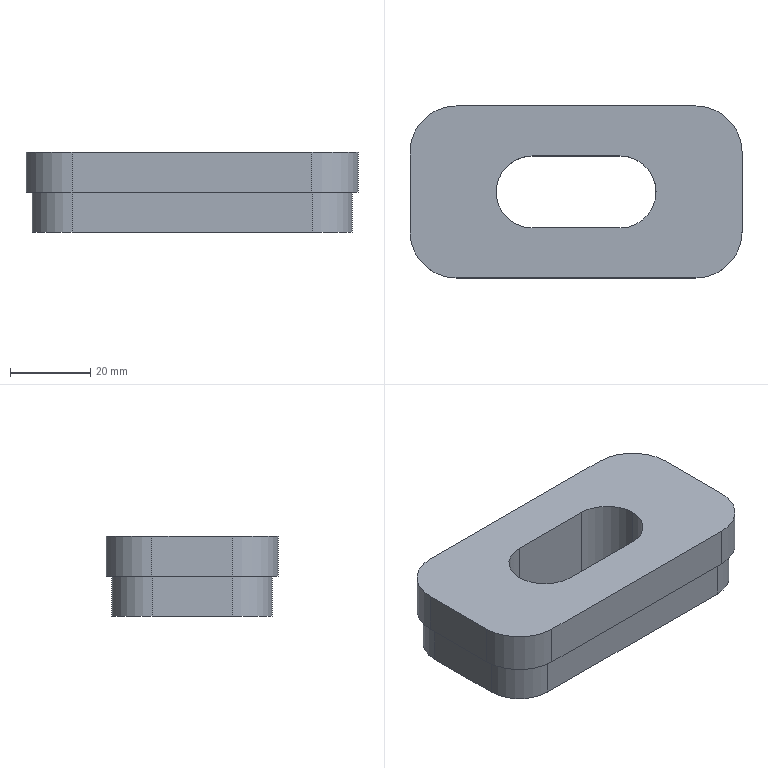Part | SolidWorks | features BaseBody 1 | 1 solid | 24 faces | box 83 x 43 x 20 mm | volume 52687 mm3 | plane 13 | cylinder 11 | commonest cylinder face diameters 20 x4 23 x4 18 x3
STEP:
#1=CARTESIAN_POINT('',(20.,0.,0.));
#2=VERTEX_POINT('',#1);
#3=CARTESIAN_POINT('',(11.,9.,0.));
#4=VERTEX_POINT('',#3);
#5=CARTESIAN_POINT('',(11.,0.,0.));
#6=DIRECTION('',(0.,0.,1.));
#7=DIRECTION('',(1.,0.,0.));
#8=AXIS2_PLACEMENT_3D('',#5,#6,#7);
#9=CIRCLE('',#8,9.);
#10=EDGE_CURVE('',#2,#4,#9,.T.);
#11=ORIENTED_EDGE('',*,*,#10,.F.);
#12=CARTESIAN_POINT('',(20.,0.,20.));
#13=VERTEX_POINT('',#12);
#14=CARTESIAN_POINT('',(20.,0.,0.));
#15=DIRECTION('',(0.,0.,1.));
#16=VECTOR('',#15,1000.);
#17=LINE('',#14,#16);
#18=EDGE_CURVE('',#2,#13,#17,.T.);
#19=ORIENTED_EDGE('',*,*,#18,.T.);
#20=CARTESIAN_POINT('',(11.,9.,20.));
#21=VERTEX_POINT('',#20);
#22=CARTESIAN_POINT('',(11.,0.,20.));
#23=DIRECTION('',(0.,0.,-1.));
#24=DIRECTION('',(1.,0.,0.));
#25=AXIS2_PLACEMENT_3D('',#22,#23,#24);
#26=CIRCLE('',#25,9.);
#27=EDGE_CURVE('',#21,#13,#26,.T.);
#28=ORIENTED_EDGE('',*,*,#27,.F.);
#29=CARTESIAN_POINT('',(11.,9.,0.));
#30=DIRECTION('',(0.,0.,1.));
#31=VECTOR('',#30,1000.);
#32=LINE('',#29,#31);
#33=EDGE_CURVE('',#4,#21,#32,.T.);
#34=ORIENTED_EDGE('',*,*,#33,.F.);
#35=EDGE_LOOP('',(#11,#19,#28,#34));
#36=FACE_OUTER_BOUND('',#35,.T.);
#37=CARTESIAN_POINT('',(11.,0.,0.));
#38=DIRECTION('',(0.,0.,1.));
#39=DIRECTION('',(1.,0.,0.));
#40=AXIS2_PLACEMENT_3D('',#37,#38,#39);
#41=CYLINDRICAL_SURFACE('',#40,9.);
#42=ADVANCED_FACE('',(#36),#41,.F.);
#43=CARTESIAN_POINT('',(11.,-9.,20.));
#44=VERTEX_POINT('',#43);
#45=CARTESIAN_POINT('',(-11.,-9.,20.));
#46=VERTEX_POINT('',#45);
#47=CARTESIAN_POINT('',(0.,-9.,20.));
#48=DIRECTION('',(-1.,0.,0.));
#49=VECTOR('',#48,1000.);
#50=LINE('',#47,#49);
#51=EDGE_CURVE('',#44,#46,#50,.T.);
#52=ORIENTED_EDGE('',*,*,#51,.T.);
#53=CARTESIAN_POINT('',(-11.,9.,20.));
#54=VERTEX_POINT('',#53);
#55=CARTESIAN_POINT('',(-11.,0.,20.));
#56=DIRECTION('',(0.,0.,-1.));
#57=DIRECTION('',(1.,0.,0.));
#58=AXIS2_PLACEMENT_3D('',#55,#56,#57);
#59=CIRCLE('',#58,9.);
#60=EDGE_CURVE('',#46,#54,#59,.T.);
#61=ORIENTED_EDGE('',*,*,#60,.T.);
#62=CARTESIAN_POINT('',(0.,9.,20.));
#63=DIRECTION('',(1.,0.,0.));
#64=VECTOR('',#63,1000.);
#65=LINE('',#62,#64);
#66=EDGE_CURVE('',#54,#21,#65,.T.);
#67=ORIENTED_EDGE('',*,*,#66,.T.);
#68=ORIENTED_EDGE('',*,*,#27,.T.);
#69=CARTESIAN_POINT('',(11.,0.,20.));
#70=DIRECTION('',(0.,0.,-1.));
#71=DIRECTION('',(1.,0.,0.));
#72=AXIS2_PLACEMENT_3D('',#69,#70,#71);
#73=CIRCLE('',#72,9.);
#74=EDGE_CURVE('',#13,#44,#73,.T.);
#75=ORIENTED_EDGE('',*,*,#74,.T.);
#76=EDGE_LOOP('',(#52,#61,#67,#68,#75));
#77=FACE_BOUND('',#76,.T.);
#78=CARTESIAN_POINT('',(41.5,-10.,20.));
#79=VERTEX_POINT('',#78);
#80=CARTESIAN_POINT('',(41.5,10.,20.));
#81=VERTEX_POINT('',#80);
#82=CARTESIAN_POINT('',(41.5,0.,20.));
#83=DIRECTION('',(0.,1.,0.));
#84=VECTOR('',#83,1000.);
#85=LINE('',#82,#84);
#86=EDGE_CURVE('',#79,#81,#85,.T.);
#87=ORIENTED_EDGE('',*,*,#86,.T.);
#88=CARTESIAN_POINT('',(30.,21.5,20.));
#89=VERTEX_POINT('',#88);
#90=CARTESIAN_POINT('',(30.,10.,20.));
#91=DIRECTION('',(0.,0.,1.));
#92=DIRECTION('',(1.,0.,0.));
#93=AXIS2_PLACEMENT_3D('',#90,#91,#92);
#94=CIRCLE('',#93,11.5);
#95=EDGE_CURVE('',#81,#89,#94,.T.);
#96=ORIENTED_EDGE('',*,*,#95,.T.);
#97=CARTESIAN_POINT('',(-30.,21.5,20.));
#98=VERTEX_POINT('',#97);
#99=CARTESIAN_POINT('',(0.,21.5,20.));
#100=DIRECTION('',(-1.,0.,0.));
#101=VECTOR('',#100,1000.);
#102=LINE('',#99,#101);
#103=EDGE_CURVE('',#89,#98,#102,.T.);
#104=ORIENTED_EDGE('',*,*,#103,.T.);
#105=CARTESIAN_POINT('',(-41.5,10.,20.));
#106=VERTEX_POINT('',#105);
#107=CARTESIAN_POINT('',(-30.,10.,20.));
#108=DIRECTION('',(0.,0.,1.));
#109=DIRECTION('',(1.,0.,0.));
#110=AXIS2_PLACEMENT_3D('',#107,#108,#109);
#111=CIRCLE('',#110,11.5);
#112=EDGE_CURVE('',#98,#106,#111,.T.);
#113=ORIENTED_EDGE('',*,*,#112,.T.);
#114=CARTESIAN_POINT('',(-41.5,-10.,20.));
#115=VERTEX_POINT('',#114);
#116=CARTESIAN_POINT('',(-41.5,0.,20.));
#117=DIRECTION('',(0.,-1.,0.));
#118=VECTOR('',#117,1000.);
#119=LINE('',#116,#118);
#120=EDGE_CURVE('',#106,#115,#119,.T.);
#121=ORIENTED_EDGE('',*,*,#120,.T.);
#122=CARTESIAN_POINT('',(-30.,-21.5,20.));
#123=VERTEX_POINT('',#122);
#124=CARTESIAN_POINT('',(-30.,-10.,20.));
#125=DIRECTION('',(0.,0.,1.));
#126=DIRECTION('',(1.,0.,0.));
#127=AXIS2_PLACEMENT_3D('',#124,#125,#126);
#128=CIRCLE('',#127,11.5);
#129=EDGE_CURVE('',#115,#123,#128,.T.);
#130=ORIENTED_EDGE('',*,*,#129,.T.);
#131=CARTESIAN_POINT('',(30.,-21.5,20.));
#132=VERTEX_POINT('',#131);
#133=CARTESIAN_POINT('',(0.,-21.5,20.));
#134=DIRECTION('',(1.,0.,0.));
#135=VECTOR('',#134,1000.);
#136=LINE('',#133,#135);
#137=EDGE_CURVE('',#123,#132,#136,.T.);
#138=ORIENTED_EDGE('',*,*,#137,.T.);
#139=CARTESIAN_POINT('',(30.,-10.,20.));
#140=DIRECTION('',(0.,0.,1.));
#141=DIRECTION('',(1.,0.,0.));
#142=AXIS2_PLACEMENT_3D('',#139,#140,#141);
#143=CIRCLE('',#142,11.5);
#144=EDGE_CURVE('',#132,#79,#143,.T.);
#145=ORIENTED_EDGE('',*,*,#144,.T.);
#146=EDGE_LOOP('',(#87,#96,#104,#113,#121,#130,#138,#145));
#147=FACE_OUTER_BOUND('',#146,.T.);
#148=CARTESIAN_POINT('',(0.,0.,20.));
#149=DIRECTION('',(0.,0.,1.));
#150=DIRECTION('',(1.,0.,0.));
#151=AXIS2_PLACEMENT_3D('',#148,#149,#150);
#152=PLANE('',#151);
#153=ADVANCED_FACE('',(#77,#147),#152,.T.);
#154=CARTESIAN_POINT('',(-11.,9.,0.));
#155=VERTEX_POINT('',#154);
#156=CARTESIAN_POINT('',(-11.,9.,0.));
#157=DIRECTION('',(0.,0.,-1.));
#158=VECTOR('',#157,1000.);
#159=LINE('',#156,#158);
#160=EDGE_CURVE('',#54,#155,#159,.T.);
#161=ORIENTED_EDGE('',*,*,#160,.F.);
#162=ORIENTED_EDGE('',*,*,#60,.F.);
#163=CARTESIAN_POINT('',(-11.,-9.,0.));
#164=VERTEX_POINT('',#163);
#165=CARTESIAN_POINT('',(-11.,-9.,0.));
#166=DIRECTION('',(0.,0.,1.));
#167=VECTOR('',#166,1000.);
#168=LINE('',#165,#167);
#169=EDGE_CURVE('',#164,#46,#168,.T.);
#170=ORIENTED_EDGE('',*,*,#169,.F.);
#171=CARTESIAN_POINT('',(-11.,0.,0.));
#172=DIRECTION('',(0.,0.,1.));
#173=DIRECTION('',(1.,0.,0.));
#174=AXIS2_PLACEMENT_3D('',#171,#172,#173);
#175=CIRCLE('',#174,9.);
#176=EDGE_CURVE('',#155,#164,#175,.T.);
#177=ORIENTED_EDGE('',*,*,#176,.F.);
#178=EDGE_LOOP('',(#161,#162,#170,#177));
#179=FACE_OUTER_BOUND('',#178,.T.);
#180=CARTESIAN_POINT('',(-11.,0.,0.));
#181=DIRECTION('',(0.,0.,1.));
#182=DIRECTION('',(1.,0.,0.));
#183=AXIS2_PLACEMENT_3D('',#180,#181,#182);
#184=CYLINDRICAL_SURFACE('',#183,9.);
#185=ADVANCED_FACE('',(#179),#184,.F.);
#186=ORIENTED_EDGE('',*,*,#51,.F.);
#187=CARTESIAN_POINT('',(11.,-9.,0.));
#188=VERTEX_POINT('',#187);
#189=CARTESIAN_POINT('',(11.,-9.,9.25));
#190=DIRECTION('',(0.,0.,-1.));
#191=VECTOR('',#190,1000.);
#192=LINE('',#189,#191);
#193=EDGE_CURVE('',#44,#188,#192,.T.);
#194=ORIENTED_EDGE('',*,*,#193,.T.);
#195=CARTESIAN_POINT('',(0.,-9.,0.));
#196=DIRECTION('',(-1.,0.,0.));
#197=VECTOR('',#196,1000.);
#198=LINE('',#195,#197);
#199=EDGE_CURVE('',#188,#164,#198,.T.);
#200=ORIENTED_EDGE('',*,*,#199,.T.);
#201=ORIENTED_EDGE('',*,*,#169,.T.);
#202=EDGE_LOOP('',(#186,#194,#200,#201));
#203=FACE_OUTER_BOUND('',#202,.T.);
#204=CARTESIAN_POINT('',(0.,-9.,9.25));
#205=DIRECTION('',(0.,1.,0.));
#206=DIRECTION('',(0.,0.,1.));
#207=AXIS2_PLACEMENT_3D('',#204,#205,#206);
#208=PLANE('',#207);
#209=ADVANCED_FACE('',(#203),#208,.T.);
#210=ORIENTED_EDGE('',*,*,#18,.F.);
#211=CARTESIAN_POINT('',(11.,0.,0.));
#212=DIRECTION('',(0.,0.,1.));
#213=DIRECTION('',(1.,0.,0.));
#214=AXIS2_PLACEMENT_3D('',#211,#212,#213);
#215=CIRCLE('',#214,9.);
#216=EDGE_CURVE('',#188,#2,#215,.T.);
#217=ORIENTED_EDGE('',*,*,#216,.F.);
#218=ORIENTED_EDGE('',*,*,#193,.F.);
#219=ORIENTED_EDGE('',*,*,#74,.F.);
#220=EDGE_LOOP('',(#210,#217,#218,#219));
#221=FACE_OUTER_BOUND('',#220,.T.);
#222=CARTESIAN_POINT('',(11.,0.,0.));
#223=DIRECTION('',(0.,0.,1.));
#224=DIRECTION('',(1.,0.,0.));
#225=AXIS2_PLACEMENT_3D('',#222,#223,#224);
#226=CYLINDRICAL_SURFACE('',#225,9.);
#227=ADVANCED_FACE('',(#221),#226,.F.);
#228=ORIENTED_EDGE('',*,*,#33,.T.);
#229=ORIENTED_EDGE('',*,*,#66,.F.);
#230=ORIENTED_EDGE('',*,*,#160,.T.);
#231=CARTESIAN_POINT('',(0.,9.,0.));
#232=DIRECTION('',(-1.,0.,0.));
#233=VECTOR('',#232,1000.);
#234=LINE('',#231,#233);
#235=EDGE_CURVE('',#4,#155,#234,.T.);
#236=ORIENTED_EDGE('',*,*,#235,.F.);
#237=EDGE_LOOP('',(#228,#229,#230,#236));
#238=FACE_OUTER_BOUND('',#237,.T.);
#239=CARTESIAN_POINT('',(0.,9.,9.25));
#240=DIRECTION('',(0.,1.,0.));
#241=DIRECTION('',(0.,0.,1.));
#242=AXIS2_PLACEMENT_3D('',#239,#240,#241);
#243=PLANE('',#242);
#244=ADVANCED_FACE('',(#238),#243,.F.);
#245=CARTESIAN_POINT('',(30.,21.5,10.));
#246=VERTEX_POINT('',#245);
#247=CARTESIAN_POINT('',(30.,21.5,10.));
#248=DIRECTION('',(0.,0.,1.));
#249=VECTOR('',#248,1000.);
#250=LINE('',#247,#249);
#251=EDGE_CURVE('',#246,#89,#250,.T.);
#252=ORIENTED_EDGE('',*,*,#251,.T.);
#253=ORIENTED_EDGE('',*,*,#95,.F.);
#254=CARTESIAN_POINT('',(41.5,10.,10.));
#255=VERTEX_POINT('',#254);
#256=CARTESIAN_POINT('',(41.5,10.,10.));
#257=DIRECTION('',(0.,0.,-1.));
#258=VECTOR('',#257,1000.);
#259=LINE('',#256,#258);
#260=EDGE_CURVE('',#81,#255,#259,.T.);
#261=ORIENTED_EDGE('',*,*,#260,.T.);
#262=CARTESIAN_POINT('',(30.,10.,10.));
#263=DIRECTION('',(0.,0.,1.));
#264=DIRECTION('',(1.,0.,0.));
#265=AXIS2_PLACEMENT_3D('',#262,#263,#264);
#266=CIRCLE('',#265,11.5);
#267=EDGE_CURVE('',#255,#246,#266,.T.);
#268=ORIENTED_EDGE('',*,*,#267,.T.);
#269=EDGE_LOOP('',(#252,#253,#261,#268));
#270=FACE_OUTER_BOUND('',#269,.T.);
#271=CARTESIAN_POINT('',(30.,10.,10.));
#272=DIRECTION('',(0.,0.,1.));
#273=DIRECTION('',(1.,0.,0.));
#274=AXIS2_PLACEMENT_3D('',#271,#272,#273);
#275=CYLINDRICAL_SURFACE('',#274,11.5);
#276=ADVANCED_FACE('',(#270),#275,.T.);
#277=ORIENTED_EDGE('',*,*,#260,.F.);
#278=ORIENTED_EDGE('',*,*,#86,.F.);
#279=CARTESIAN_POINT('',(41.5,-10.,10.));
#280=VERTEX_POINT('',#279);
#281=CARTESIAN_POINT('',(41.5,-10.,15.));
#282=DIRECTION('',(0.,0.,-1.));
#283=VECTOR('',#282,1000.);
#284=LINE('',#281,#283);
#285=EDGE_CURVE('',#79,#280,#284,.T.);
#286=ORIENTED_EDGE('',*,*,#285,.T.);
#287=CARTESIAN_POINT('',(41.5,0.,10.));
#288=DIRECTION('',(0.,1.,0.));
#289=VECTOR('',#288,1000.);
#290=LINE('',#287,#289);
#291=EDGE_CURVE('',#280,#255,#290,.T.);
#292=ORIENTED_EDGE('',*,*,#291,.T.);
#293=EDGE_LOOP('',(#277,#278,#286,#292));
#294=FACE_OUTER_BOUND('',#293,.T.);
#295=CARTESIAN_POINT('',(41.5,0.,15.));
#296=DIRECTION('',(1.,0.,0.));
#297=DIRECTION('',(0.,0.,-1.));
#298=AXIS2_PLACEMENT_3D('',#295,#296,#297);
#299=PLANE('',#298);
#300=ADVANCED_FACE('',(#294),#299,.T.);
#301=ORIENTED_EDGE('',*,*,#285,.F.);
#302=ORIENTED_EDGE('',*,*,#144,.F.);
#303=CARTESIAN_POINT('',(30.,-21.5,10.));
#304=VERTEX_POINT('',#303);
#305=CARTESIAN_POINT('',(30.,-21.5,10.));
#306=DIRECTION('',(0.,0.,-1.));
#307=VECTOR('',#306,1000.);
#308=LINE('',#305,#307);
#309=EDGE_CURVE('',#132,#304,#308,.T.);
#310=ORIENTED_EDGE('',*,*,#309,.T.);
#311=CARTESIAN_POINT('',(30.,-10.,10.));
#312=DIRECTION('',(0.,0.,1.));
#313=DIRECTION('',(1.,0.,0.));
#314=AXIS2_PLACEMENT_3D('',#311,#312,#313);
#315=CIRCLE('',#314,11.5);
#316=EDGE_CURVE('',#304,#280,#315,.T.);
#317=ORIENTED_EDGE('',*,*,#316,.T.);
#318=EDGE_LOOP('',(#301,#302,#310,#317));
#319=FACE_OUTER_BOUND('',#318,.T.);
#320=CARTESIAN_POINT('',(30.,-10.,10.));
#321=DIRECTION('',(0.,0.,1.));
#322=DIRECTION('',(1.,0.,0.));
#323=AXIS2_PLACEMENT_3D('',#320,#321,#322);
#324=CYLINDRICAL_SURFACE('',#323,11.5);
#325=ADVANCED_FACE('',(#319),#324,.T.);
#326=CARTESIAN_POINT('',(-30.,-21.5,10.));
#327=VERTEX_POINT('',#326);
#328=CARTESIAN_POINT('',(0.,-21.5,10.));
#329=DIRECTION('',(-1.,0.,0.));
#330=VECTOR('',#329,1000.);
#331=LINE('',#328,#330);
#332=EDGE_CURVE('',#304,#327,#331,.T.);
#333=ORIENTED_EDGE('',*,*,#332,.F.);
#334=ORIENTED_EDGE('',*,*,#309,.F.);
#335=ORIENTED_EDGE('',*,*,#137,.F.);
#336=CARTESIAN_POINT('',(-30.,-21.5,15.));
#337=DIRECTION('',(0.,0.,1.));
#338=VECTOR('',#337,1000.);
#339=LINE('',#336,#338);
#340=EDGE_CURVE('',#327,#123,#339,.T.);
#341=ORIENTED_EDGE('',*,*,#340,.F.);
#342=EDGE_LOOP('',(#333,#334,#335,#341));
#343=FACE_OUTER_BOUND('',#342,.T.);
#344=CARTESIAN_POINT('',(0.,-21.5,15.));
#345=DIRECTION('',(0.,1.,0.));
#346=DIRECTION('',(0.,0.,1.));
#347=AXIS2_PLACEMENT_3D('',#344,#345,#346);
#348=PLANE('',#347);
#349=ADVANCED_FACE('',(#343),#348,.F.);
#350=ORIENTED_EDGE('',*,*,#340,.T.);
#351=ORIENTED_EDGE('',*,*,#129,.F.);
#352=CARTESIAN_POINT('',(-41.5,-10.,10.));
#353=VERTEX_POINT('',#352);
#354=CARTESIAN_POINT('',(-41.5,-10.,10.));
#355=DIRECTION('',(0.,0.,-1.));
#356=VECTOR('',#355,1000.);
#357=LINE('',#354,#356);
#358=EDGE_CURVE('',#115,#353,#357,.T.);
#359=ORIENTED_EDGE('',*,*,#358,.T.);
#360=CARTESIAN_POINT('',(-30.,-10.,10.));
#361=DIRECTION('',(0.,0.,1.));
#362=DIRECTION('',(1.,0.,0.));
#363=AXIS2_PLACEMENT_3D('',#360,#361,#362);
#364=CIRCLE('',#363,11.5);
#365=EDGE_CURVE('',#353,#327,#364,.T.);
#366=ORIENTED_EDGE('',*,*,#365,.T.);
#367=EDGE_LOOP('',(#350,#351,#359,#366));
#368=FACE_OUTER_BOUND('',#367,.T.);
#369=CARTESIAN_POINT('',(-30.,-10.,10.));
#370=DIRECTION('',(0.,0.,1.));
#371=DIRECTION('',(1.,0.,0.));
#372=AXIS2_PLACEMENT_3D('',#369,#370,#371);
#373=CYLINDRICAL_SURFACE('',#372,11.5);
#374=ADVANCED_FACE('',(#368),#373,.T.);
#375=CARTESIAN_POINT('',(-41.5,10.,10.));
#376=VERTEX_POINT('',#375);
#377=CARTESIAN_POINT('',(-41.5,0.,10.));
#378=DIRECTION('',(0.,1.,0.));
#379=VECTOR('',#378,1000.);
#380=LINE('',#377,#379);
#381=EDGE_CURVE('',#353,#376,#380,.T.);
#382=ORIENTED_EDGE('',*,*,#381,.F.);
#383=ORIENTED_EDGE('',*,*,#358,.F.);
#384=ORIENTED_EDGE('',*,*,#120,.F.);
#385=CARTESIAN_POINT('',(-41.5,10.,15.));
#386=DIRECTION('',(0.,0.,1.));
#387=VECTOR('',#386,1000.);
#388=LINE('',#385,#387);
#389=EDGE_CURVE('',#376,#106,#388,.T.);
#390=ORIENTED_EDGE('',*,*,#389,.F.);
#391=EDGE_LOOP('',(#382,#383,#384,#390));
#392=FACE_OUTER_BOUND('',#391,.T.);
#393=CARTESIAN_POINT('',(-41.5,0.,15.));
#394=DIRECTION('',(1.,0.,0.));
#395=DIRECTION('',(0.,0.,-1.));
#396=AXIS2_PLACEMENT_3D('',#393,#394,#395);
#397=PLANE('',#396);
#398=ADVANCED_FACE('',(#392),#397,.F.);
#399=ORIENTED_EDGE('',*,*,#389,.T.);
#400=ORIENTED_EDGE('',*,*,#112,.F.);
#401=CARTESIAN_POINT('',(-30.,21.5,10.));
#402=VERTEX_POINT('',#401);
#403=CARTESIAN_POINT('',(-30.,21.5,10.));
#404=DIRECTION('',(0.,0.,-1.));
#405=VECTOR('',#404,1000.);
#406=LINE('',#403,#405);
#407=EDGE_CURVE('',#98,#402,#406,.T.);
#408=ORIENTED_EDGE('',*,*,#407,.T.);
#409=CARTESIAN_POINT('',(-30.,10.,10.));
#410=DIRECTION('',(0.,0.,1.));
#411=DIRECTION('',(1.,0.,0.));
#412=AXIS2_PLACEMENT_3D('',#409,#410,#411);
#413=CIRCLE('',#412,11.5);
#414=EDGE_CURVE('',#402,#376,#413,.T.);
#415=ORIENTED_EDGE('',*,*,#414,.T.);
#416=EDGE_LOOP('',(#399,#400,#408,#415));
#417=FACE_OUTER_BOUND('',#416,.T.);
#418=CARTESIAN_POINT('',(-30.,10.,10.));
#419=DIRECTION('',(0.,0.,1.));
#420=DIRECTION('',(1.,0.,0.));
#421=AXIS2_PLACEMENT_3D('',#418,#419,#420);
#422=CYLINDRICAL_SURFACE('',#421,11.5);
#423=ADVANCED_FACE('',(#417),#422,.T.);
#424=ORIENTED_EDGE('',*,*,#407,.F.);
#425=ORIENTED_EDGE('',*,*,#103,.F.);
#426=ORIENTED_EDGE('',*,*,#251,.F.);
#427=CARTESIAN_POINT('',(0.,21.5,10.));
#428=DIRECTION('',(-1.,0.,0.));
#429=VECTOR('',#428,1000.);
#430=LINE('',#427,#429);
#431=EDGE_CURVE('',#246,#402,#430,.T.);
#432=ORIENTED_EDGE('',*,*,#431,.T.);
#433=EDGE_LOOP('',(#424,#425,#426,#432));
#434=FACE_OUTER_BOUND('',#433,.T.);
#435=CARTESIAN_POINT('',(0.,21.5,15.));
#436=DIRECTION('',(0.,1.,0.));
#437=DIRECTION('',(0.,0.,1.));
#438=AXIS2_PLACEMENT_3D('',#435,#436,#437);
#439=PLANE('',#438);
#440=ADVANCED_FACE('',(#434),#439,.T.);
#441=ORIENTED_EDGE('',*,*,#216,.T.);
#442=ORIENTED_EDGE('',*,*,#10,.T.);
#443=ORIENTED_EDGE('',*,*,#235,.T.);
#444=ORIENTED_EDGE('',*,*,#176,.T.);
#445=ORIENTED_EDGE('',*,*,#199,.F.);
#446=EDGE_LOOP('',(#441,#442,#443,#444,#445));
#447=FACE_BOUND('',#446,.T.);
#448=CARTESIAN_POINT('',(30.,-20.,0.));
#449=VERTEX_POINT('',#448);
#450=CARTESIAN_POINT('',(40.,-10.,0.));
#451=VERTEX_POINT('',#450);
#452=CARTESIAN_POINT('',(30.,-10.,0.));
#453=DIRECTION('',(0.,0.,1.));
#454=DIRECTION('',(-1.,0.,0.));
#455=AXIS2_PLACEMENT_3D('',#452,#453,#454);
#456=CIRCLE('',#455,10.);
#457=EDGE_CURVE('',#449,#451,#456,.T.);
#458=ORIENTED_EDGE('',*,*,#457,.F.);
#459=CARTESIAN_POINT('',(-30.,-20.,0.));
#460=VERTEX_POINT('',#459);
#461=CARTESIAN_POINT('',(0.,-20.,0.));
#462=DIRECTION('',(1.,0.,0.));
#463=VECTOR('',#462,1000.);
#464=LINE('',#461,#463);
#465=EDGE_CURVE('',#460,#449,#464,.T.);
#466=ORIENTED_EDGE('',*,*,#465,.F.);
#467=CARTESIAN_POINT('',(-40.,-10.,0.));
#468=VERTEX_POINT('',#467);
#469=CARTESIAN_POINT('',(-30.,-10.,0.));
#470=DIRECTION('',(0.,0.,1.));
#471=DIRECTION('',(-1.,0.,0.));
#472=AXIS2_PLACEMENT_3D('',#469,#470,#471);
#473=CIRCLE('',#472,10.);
#474=EDGE_CURVE('',#468,#460,#473,.T.);
#475=ORIENTED_EDGE('',*,*,#474,.F.);
#476=CARTESIAN_POINT('',(-40.,10.,0.));
#477=VERTEX_POINT('',#476);
#478=CARTESIAN_POINT('',(-40.,0.,0.));
#479=DIRECTION('',(0.,-1.,0.));
#480=VECTOR('',#479,1000.);
#481=LINE('',#478,#480);
#482=EDGE_CURVE('',#477,#468,#481,.T.);
#483=ORIENTED_EDGE('',*,*,#482,.F.);
#484=CARTESIAN_POINT('',(-30.,20.,0.));
#485=VERTEX_POINT('',#484);
#486=CARTESIAN_POINT('',(-30.,10.,0.));
#487=DIRECTION('',(0.,0.,1.));
#488=DIRECTION('',(-1.,0.,0.));
#489=AXIS2_PLACEMENT_3D('',#486,#487,#488);
#490=CIRCLE('',#489,10.);
#491=EDGE_CURVE('',#485,#477,#490,.T.);
#492=ORIENTED_EDGE('',*,*,#491,.F.);
#493=CARTESIAN_POINT('',(30.,20.,0.));
#494=VERTEX_POINT('',#493);
#495=CARTESIAN_POINT('',(0.,20.,0.));
#496=DIRECTION('',(-1.,0.,0.));
#497=VECTOR('',#496,1000.);
#498=LINE('',#495,#497);
#499=EDGE_CURVE('',#494,#485,#498,.T.);
#500=ORIENTED_EDGE('',*,*,#499,.F.);
#501=CARTESIAN_POINT('',(40.,10.,0.));
#502=VERTEX_POINT('',#501);
#503=CARTESIAN_POINT('',(30.,10.,0.));
#504=DIRECTION('',(0.,0.,1.));
#505=DIRECTION('',(-1.,0.,0.));
#506=AXIS2_PLACEMENT_3D('',#503,#504,#505);
#507=CIRCLE('',#506,10.);
#508=EDGE_CURVE('',#502,#494,#507,.T.);
#509=ORIENTED_EDGE('',*,*,#508,.F.);
#510=CARTESIAN_POINT('',(40.,0.,0.));
#511=DIRECTION('',(0.,1.,0.));
#512=VECTOR('',#511,1000.);
#513=LINE('',#510,#512);
#514=EDGE_CURVE('',#451,#502,#513,.T.);
#515=ORIENTED_EDGE('',*,*,#514,.F.);
#516=EDGE_LOOP('',(#458,#466,#475,#483,#492,#500,#509,#515));
#517=FACE_OUTER_BOUND('',#516,.T.);
#518=CARTESIAN_POINT('',(0.,0.,0.));
#519=DIRECTION('',(0.,0.,1.));
#520=DIRECTION('',(1.,0.,0.));
#521=AXIS2_PLACEMENT_3D('',#518,#519,#520);
#522=PLANE('',#521);
#523=ADVANCED_FACE('',(#447,#517),#522,.F.);
#524=CARTESIAN_POINT('',(-40.,10.,10.));
#525=VERTEX_POINT('',#524);
#526=CARTESIAN_POINT('',(-30.,20.,10.));
#527=VERTEX_POINT('',#526);
#528=CARTESIAN_POINT('',(-30.,10.,10.));
#529=DIRECTION('',(0.,0.,-1.));
#530=DIRECTION('',(-1.,0.,0.));
#531=AXIS2_PLACEMENT_3D('',#528,#529,#530);
#532=CIRCLE('',#531,10.);
#533=EDGE_CURVE('',#525,#527,#532,.T.);
#534=ORIENTED_EDGE('',*,*,#533,.F.);
#535=CARTESIAN_POINT('',(-40.,-10.,10.));
#536=VERTEX_POINT('',#535);
#537=CARTESIAN_POINT('',(-40.,0.,10.));
#538=DIRECTION('',(0.,1.,0.));
#539=VECTOR('',#538,1000.);
#540=LINE('',#537,#539);
#541=EDGE_CURVE('',#536,#525,#540,.T.);
#542=ORIENTED_EDGE('',*,*,#541,.F.);
#543=CARTESIAN_POINT('',(-30.,-20.,10.));
#544=VERTEX_POINT('',#543);
#545=CARTESIAN_POINT('',(-30.,-10.,10.));
#546=DIRECTION('',(0.,0.,-1.));
#547=DIRECTION('',(-1.,0.,0.));
#548=AXIS2_PLACEMENT_3D('',#545,#546,#547);
#549=CIRCLE('',#548,10.);
#550=EDGE_CURVE('',#544,#536,#549,.T.);
#551=ORIENTED_EDGE('',*,*,#550,.F.);
#552=CARTESIAN_POINT('',(30.,-20.,10.));
#553=VERTEX_POINT('',#552);
#554=CARTESIAN_POINT('',(0.,-20.,10.));
#555=DIRECTION('',(-1.,0.,0.));
#556=VECTOR('',#555,1000.);
#557=LINE('',#554,#556);
#558=EDGE_CURVE('',#553,#544,#557,.T.);
#559=ORIENTED_EDGE('',*,*,#558,.F.);
#560=CARTESIAN_POINT('',(40.,-10.,10.));
#561=VERTEX_POINT('',#560);
#562=CARTESIAN_POINT('',(30.,-10.,10.));
#563=DIRECTION('',(0.,0.,-1.));
#564=DIRECTION('',(-1.,0.,0.));
#565=AXIS2_PLACEMENT_3D('',#562,#563,#564);
#566=CIRCLE('',#565,10.);
#567=EDGE_CURVE('',#561,#553,#566,.T.);
#568=ORIENTED_EDGE('',*,*,#567,.F.);
#569=CARTESIAN_POINT('',(40.,10.,10.));
#570=VERTEX_POINT('',#569);
#571=CARTESIAN_POINT('',(40.,0.,10.));
#572=DIRECTION('',(0.,-1.,0.));
#573=VECTOR('',#572,1000.);
#574=LINE('',#571,#573);
#575=EDGE_CURVE('',#570,#561,#574,.T.);
#576=ORIENTED_EDGE('',*,*,#575,.F.);
#577=CARTESIAN_POINT('',(30.,20.,10.));
#578=VERTEX_POINT('',#577);
#579=CARTESIAN_POINT('',(30.,10.,10.));
#580=DIRECTION('',(0.,0.,-1.));
#581=DIRECTION('',(-1.,0.,0.));
#582=AXIS2_PLACEMENT_3D('',#579,#580,#581);
#583=CIRCLE('',#582,10.);
#584=EDGE_CURVE('',#578,#570,#583,.T.);
#585=ORIENTED_EDGE('',*,*,#584,.F.);
#586=CARTESIAN_POINT('',(0.,20.,10.));
#587=DIRECTION('',(1.,0.,0.));
#588=VECTOR('',#587,1000.);
#589=LINE('',#586,#588);
#590=EDGE_CURVE('',#527,#578,#589,.T.);
#591=ORIENTED_EDGE('',*,*,#590,.F.);
#592=EDGE_LOOP('',(#534,#542,#551,#559,#568,#576,#585,#591));
#593=FACE_BOUND('',#592,.T.);
#594=ORIENTED_EDGE('',*,*,#291,.F.);
#595=ORIENTED_EDGE('',*,*,#316,.F.);
#596=ORIENTED_EDGE('',*,*,#332,.T.);
#597=ORIENTED_EDGE('',*,*,#365,.F.);
#598=ORIENTED_EDGE('',*,*,#381,.T.);
#599=ORIENTED_EDGE('',*,*,#414,.F.);
#600=ORIENTED_EDGE('',*,*,#431,.F.);
#601=ORIENTED_EDGE('',*,*,#267,.F.);
#602=EDGE_LOOP('',(#594,#595,#596,#597,#598,#599,#600,#601));
#603=FACE_OUTER_BOUND('',#602,.T.);
#604=CARTESIAN_POINT('',(0.,0.,10.));
#605=DIRECTION('',(0.,0.,1.));
#606=DIRECTION('',(1.,0.,0.));
#607=AXIS2_PLACEMENT_3D('',#604,#605,#606);
#608=PLANE('',#607);
#609=ADVANCED_FACE('',(#593,#603),#608,.F.);
#610=CARTESIAN_POINT('',(40.,10.,9.25));
#611=DIRECTION('',(0.,0.,1.));
#612=VECTOR('',#611,1000.);
#613=LINE('',#610,#612);
#614=EDGE_CURVE('',#502,#570,#613,.T.);
#615=ORIENTED_EDGE('',*,*,#614,.T.);
#616=ORIENTED_EDGE('',*,*,#575,.T.);
#617=CARTESIAN_POINT('',(40.,-10.,9.25));
#618=DIRECTION('',(0.,0.,-1.));
#619=VECTOR('',#618,1000.);
#620=LINE('',#617,#619);
#621=EDGE_CURVE('',#561,#451,#620,.T.);
#622=ORIENTED_EDGE('',*,*,#621,.T.);
#623=ORIENTED_EDGE('',*,*,#514,.T.);
#624=EDGE_LOOP('',(#615,#616,#622,#623));
#625=FACE_OUTER_BOUND('',#624,.T.);
#626=CARTESIAN_POINT('',(40.,0.,9.25));
#627=DIRECTION('',(1.,0.,0.));
#628=DIRECTION('',(0.,0.,-1.));
#629=AXIS2_PLACEMENT_3D('',#626,#627,#628);
#630=PLANE('',#629);
#631=ADVANCED_FACE('',(#625),#630,.T.);
#632=ORIENTED_EDGE('',*,*,#621,.F.);
#633=ORIENTED_EDGE('',*,*,#567,.T.);
#634=CARTESIAN_POINT('',(30.,-20.,18.5));
#635=DIRECTION('',(0.,0.,-1.));
#636=VECTOR('',#635,1000.);
#637=LINE('',#634,#636);
#638=EDGE_CURVE('',#553,#449,#637,.T.);
#639=ORIENTED_EDGE('',*,*,#638,.T.);
#640=ORIENTED_EDGE('',*,*,#457,.T.);
#641=EDGE_LOOP('',(#632,#633,#639,#640));
#642=FACE_OUTER_BOUND('',#641,.T.);
#643=CARTESIAN_POINT('',(30.,-10.,18.5));
#644=DIRECTION('',(0.,0.,-1.));
#645=DIRECTION('',(-1.,0.,0.));
#646=AXIS2_PLACEMENT_3D('',#643,#644,#645);
#647=CYLINDRICAL_SURFACE('',#646,10.);
#648=ADVANCED_FACE('',(#642),#647,.T.);
#649=ORIENTED_EDGE('',*,*,#465,.T.);
#650=ORIENTED_EDGE('',*,*,#638,.F.);
#651=ORIENTED_EDGE('',*,*,#558,.T.);
#652=CARTESIAN_POINT('',(-30.,-20.,9.25));
#653=DIRECTION('',(0.,0.,1.));
#654=VECTOR('',#653,1000.);
#655=LINE('',#652,#654);
#656=EDGE_CURVE('',#460,#544,#655,.T.);
#657=ORIENTED_EDGE('',*,*,#656,.F.);
#658=EDGE_LOOP('',(#649,#650,#651,#657));
#659=FACE_OUTER_BOUND('',#658,.T.);
#660=CARTESIAN_POINT('',(0.,-20.,9.25));
#661=DIRECTION('',(0.,1.,0.));
#662=DIRECTION('',(0.,0.,1.));
#663=AXIS2_PLACEMENT_3D('',#660,#661,#662);
#664=PLANE('',#663);
#665=ADVANCED_FACE('',(#659),#664,.F.);
#666=ORIENTED_EDGE('',*,*,#656,.T.);
#667=ORIENTED_EDGE('',*,*,#550,.T.);
#668=CARTESIAN_POINT('',(-40.,-10.,18.5));
#669=DIRECTION('',(0.,0.,-1.));
#670=VECTOR('',#669,1000.);
#671=LINE('',#668,#670);
#672=EDGE_CURVE('',#536,#468,#671,.T.);
#673=ORIENTED_EDGE('',*,*,#672,.T.);
#674=ORIENTED_EDGE('',*,*,#474,.T.);
#675=EDGE_LOOP('',(#666,#667,#673,#674));
#676=FACE_OUTER_BOUND('',#675,.T.);
#677=CARTESIAN_POINT('',(-30.,-10.,18.5));
#678=DIRECTION('',(0.,0.,-1.));
#679=DIRECTION('',(-1.,0.,0.));
#680=AXIS2_PLACEMENT_3D('',#677,#678,#679);
#681=CYLINDRICAL_SURFACE('',#680,10.);
#682=ADVANCED_FACE('',(#676),#681,.T.);
#683=ORIENTED_EDGE('',*,*,#482,.T.);
#684=ORIENTED_EDGE('',*,*,#672,.F.);
#685=ORIENTED_EDGE('',*,*,#541,.T.);
#686=CARTESIAN_POINT('',(-40.,10.,9.25));
#687=DIRECTION('',(0.,0.,1.));
#688=VECTOR('',#687,1000.);
#689=LINE('',#686,#688);
#690=EDGE_CURVE('',#477,#525,#689,.T.);
#691=ORIENTED_EDGE('',*,*,#690,.F.);
#692=EDGE_LOOP('',(#683,#684,#685,#691));
#693=FACE_OUTER_BOUND('',#692,.T.);
#694=CARTESIAN_POINT('',(-40.,0.,9.25));
#695=DIRECTION('',(1.,0.,0.));
#696=DIRECTION('',(0.,0.,-1.));
#697=AXIS2_PLACEMENT_3D('',#694,#695,#696);
#698=PLANE('',#697);
#699=ADVANCED_FACE('',(#693),#698,.F.);
#700=ORIENTED_EDGE('',*,*,#690,.T.);
#701=ORIENTED_EDGE('',*,*,#533,.T.);
#702=CARTESIAN_POINT('',(-30.,20.,18.5));
#703=DIRECTION('',(0.,0.,-1.));
#704=VECTOR('',#703,1000.);
#705=LINE('',#702,#704);
#706=EDGE_CURVE('',#527,#485,#705,.T.);
#707=ORIENTED_EDGE('',*,*,#706,.T.);
#708=ORIENTED_EDGE('',*,*,#491,.T.);
#709=EDGE_LOOP('',(#700,#701,#707,#708));
#710=FACE_OUTER_BOUND('',#709,.T.);
#711=CARTESIAN_POINT('',(-30.,10.,18.5));
#712=DIRECTION('',(0.,0.,-1.));
#713=DIRECTION('',(-1.,0.,0.));
#714=AXIS2_PLACEMENT_3D('',#711,#712,#713);
#715=CYLINDRICAL_SURFACE('',#714,10.);
#716=ADVANCED_FACE('',(#710),#715,.T.);
#717=ORIENTED_EDGE('',*,*,#706,.F.);
#718=ORIENTED_EDGE('',*,*,#590,.T.);
#719=CARTESIAN_POINT('',(30.,20.,9.25));
#720=DIRECTION('',(0.,0.,-1.));
#721=VECTOR('',#720,1000.);
#722=LINE('',#719,#721);
#723=EDGE_CURVE('',#578,#494,#722,.T.);
#724=ORIENTED_EDGE('',*,*,#723,.T.);
#725=ORIENTED_EDGE('',*,*,#499,.T.);
#726=EDGE_LOOP('',(#717,#718,#724,#725));
#727=FACE_OUTER_BOUND('',#726,.T.);
#728=CARTESIAN_POINT('',(0.,20.,9.25));
#729=DIRECTION('',(0.,1.,0.));
#730=DIRECTION('',(0.,0.,1.));
#731=AXIS2_PLACEMENT_3D('',#728,#729,#730);
#732=PLANE('',#731);
#733=ADVANCED_FACE('',(#727),#732,.T.);
#734=ORIENTED_EDGE('',*,*,#723,.F.);
#735=ORIENTED_EDGE('',*,*,#584,.T.);
#736=ORIENTED_EDGE('',*,*,#614,.F.);
#737=ORIENTED_EDGE('',*,*,#508,.T.);
#738=EDGE_LOOP('',(#734,#735,#736,#737));
#739=FACE_OUTER_BOUND('',#738,.T.);
#740=CARTESIAN_POINT('',(30.,10.,18.5));
#741=DIRECTION('',(0.,0.,-1.));
#742=DIRECTION('',(-1.,0.,0.));
#743=AXIS2_PLACEMENT_3D('',#740,#741,#742);
#744=CYLINDRICAL_SURFACE('',#743,10.);
#745=ADVANCED_FACE('',(#739),#744,.T.);
#746=CLOSED_SHELL('',(#42,#153,#185,#209,#227,#244,#276,#300,#325,#349,#374,#398,#423,#440,#523,#609,#631,#648,#665,#682,#699,#716,#733,#745));
#747=MANIFOLD_SOLID_BREP('',#746);
#748=CARTESIAN_POINT('',(0.,0.,0.));
#749=DIRECTION('',(0.,0.,1.));
#750=DIRECTION('',(1.,0.,0.));
#751=AXIS2_PLACEMENT_3D('',#748,#749,#750);
#752=(LENGTH_UNIT()NAMED_UNIT(*)SI_UNIT(.MILLI.,.METRE.));
#753=UNCERTAINTY_MEASURE_WITH_UNIT(LENGTH_MEASURE(0.00001),#752,'','');
#754=(NAMED_UNIT(*)PLANE_ANGLE_UNIT()SI_UNIT($,.RADIAN.));
#755=(NAMED_UNIT(*)SI_UNIT($,.STERADIAN.)SOLID_ANGLE_UNIT());
#756=(GEOMETRIC_REPRESENTATION_CONTEXT(3)GLOBAL_UNCERTAINTY_ASSIGNED_CONTEXT((#753))GLOBAL_UNIT_ASSIGNED_CONTEXT((#752,#754,#755))REPRESENTATION_CONTEXT('',''));
#757=ADVANCED_BREP_SHAPE_REPRESENTATION('',(#747,#751),#756);